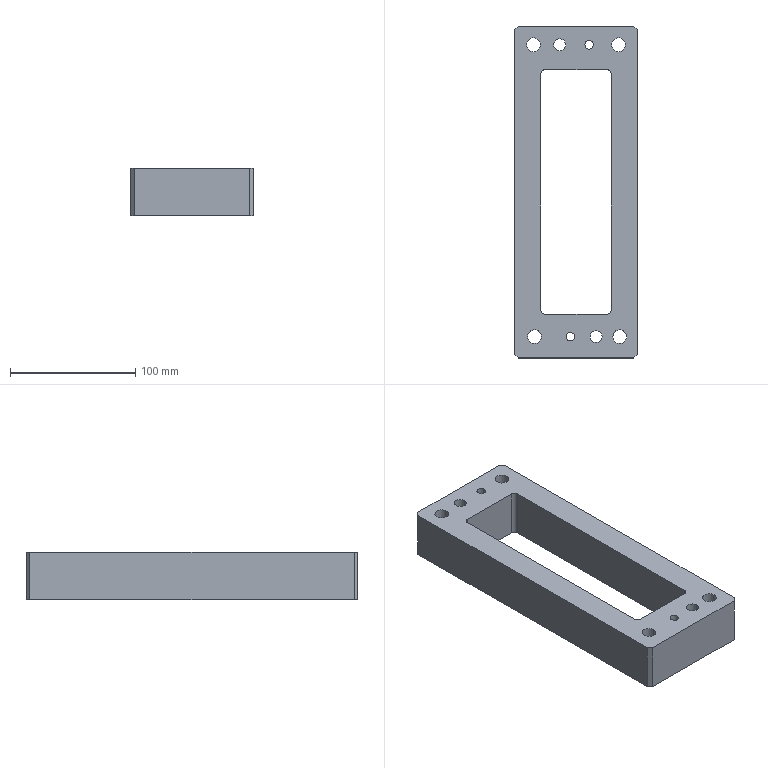Part | STEP file | 1_id170_x_t | 1 solid | 34 faces | box 98 x 265 x 38.1 mm | volume 540767 mm3 | plane 18 | cylinder 16 | commonest cylinder face diameters 6 x4 11 x4 18 x4 6.8 x2 9.525 x2